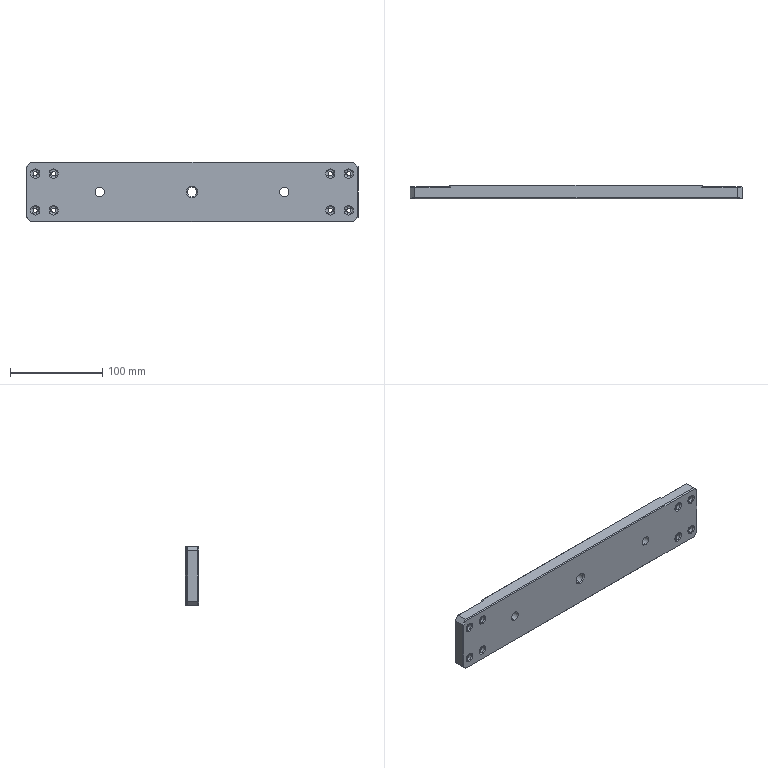Part | SolidWorks | features HoleWzd 3, ICE 3, Chamfer 2, Extrusion 1 | 1 solid | 136 faces | box 360 x 15 x 65 mm | volume 330070 mm3 | plane 54 | cylinder 46 | cone 36 | commonest cylinder face diameters 4.5 x16 8 x16 3.3 x4 10 x4 20 x4 10.5 x2